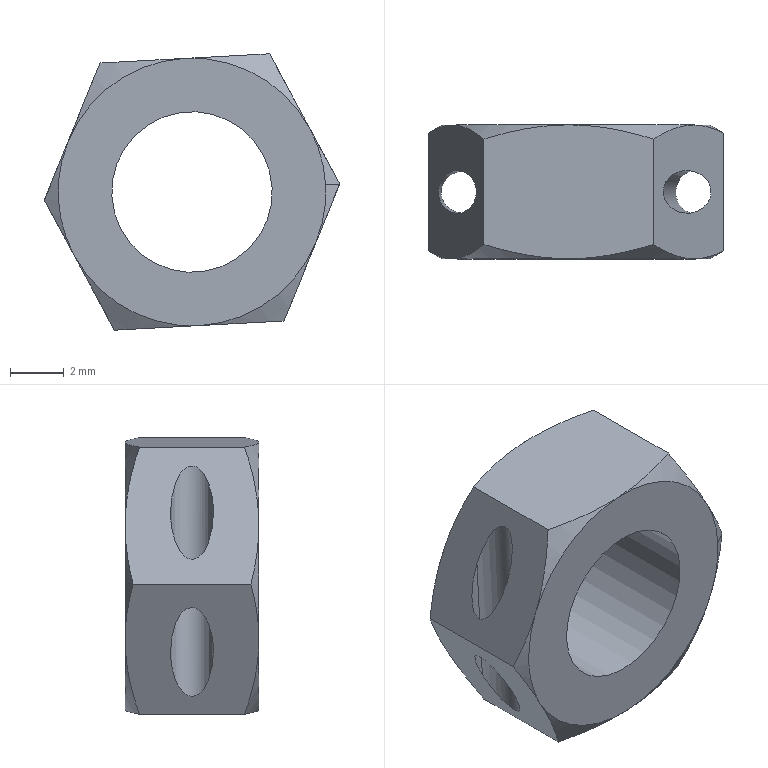Part | SolidWorks | features BaseBody 1 | 1 solid | 30 faces | box 11.034 x 5 x 10.33 mm | volume 267.643 mm3 | cone 16 | plane 8 | cylinder 6 | commonest cylinder face diameters 1.6 x4 6 x2
STEP:
#1=CARTESIAN_POINT('',(303.735,265.5,-2.369));
#2=VERTEX_POINT('',#1);
#3=CARTESIAN_POINT('',(303.735,267.1,-2.369));
#4=VERTEX_POINT('',#3);
#5=CARTESIAN_POINT('',(303.735,265.5,-2.369));
#6=CARTESIAN_POINT('',(305.148,265.5,1.117));
#7=CARTESIAN_POINT('',(305.148,267.1,1.117));
#8=CARTESIAN_POINT('',(303.735,267.1,-2.369));
#9=(BOUNDED_CURVE()B_SPLINE_CURVE(3,(#5,#6,#7,#8),.UNSPECIFIED.,.F.,.F.)B_SPLINE_CURVE_WITH_KNOTS((4,4),(4.712,7.854),.UNSPECIFIED.)CURVE()GEOMETRIC_REPRESENTATION_ITEM()RATIONAL_B_SPLINE_CURVE((1.,0.3333,0.3333,1.))REPRESENTATION_ITEM(''));
#10=EDGE_CURVE('',#2,#4,#9,.T.);
#11=ORIENTED_EDGE('',*,*,#10,.F.);
#12=CARTESIAN_POINT('',(303.452,265.5,2.835));
#13=VERTEX_POINT('',#12);
#14=CARTESIAN_POINT('',(303.865,265.5,-4.759));
#15=DIRECTION('',(-0.05426,0.,0.9985));
#16=VECTOR('',#15,1000.);
#17=LINE('',#14,#16);
#18=EDGE_CURVE('',#2,#13,#17,.T.);
#19=ORIENTED_EDGE('',*,*,#18,.T.);
#20=CARTESIAN_POINT('',(303.452,267.1,2.835));
#21=VERTEX_POINT('',#20);
#22=CARTESIAN_POINT('',(303.452,267.1,2.835));
#23=CARTESIAN_POINT('',(305.235,267.1,-0.4764));
#24=CARTESIAN_POINT('',(305.235,265.5,-0.4764));
#25=CARTESIAN_POINT('',(303.452,265.5,2.835));
#26=(BOUNDED_CURVE()B_SPLINE_CURVE(3,(#22,#23,#24,#25),.UNSPECIFIED.,.F.,.F.)B_SPLINE_CURVE_WITH_KNOTS((4,4),(1.571,4.712),.UNSPECIFIED.)CURVE()GEOMETRIC_REPRESENTATION_ITEM()RATIONAL_B_SPLINE_CURVE((1.,0.3333,0.3333,1.))REPRESENTATION_ITEM(''));
#27=EDGE_CURVE('',#21,#13,#26,.T.);
#28=ORIENTED_EDGE('',*,*,#27,.F.);
#29=CARTESIAN_POINT('',(303.865,267.1,-4.759));
#30=DIRECTION('',(-0.05426,0.,0.9985));
#31=VECTOR('',#30,1000.);
#32=LINE('',#29,#31);
#33=EDGE_CURVE('',#4,#21,#32,.T.);
#34=ORIENTED_EDGE('',*,*,#33,.F.);
#35=EDGE_LOOP('',(#11,#19,#28,#34));
#36=FACE_OUTER_BOUND('',#35,.T.);
#37=CARTESIAN_POINT('',(303.865,266.3,-4.759));
#38=DIRECTION('',(-0.05426,0.,0.9985));
#39=DIRECTION('',(0.,1.,0.));
#40=AXIS2_PLACEMENT_3D('',#37,#38,#39);
#41=CYLINDRICAL_SURFACE('',#40,0.8);
#42=ADVANCED_FACE('',(#36),#41,.F.);
#43=CARTESIAN_POINT('',(295.148,265.5,-2.835));
#44=VERTEX_POINT('',#43);
#45=CARTESIAN_POINT('',(295.148,267.1,-2.835));
#46=VERTEX_POINT('',#45);
#47=CARTESIAN_POINT('',(295.148,265.5,-2.835));
#48=CARTESIAN_POINT('',(296.93,265.5,-6.147));
#49=CARTESIAN_POINT('',(296.93,267.1,-6.147));
#50=CARTESIAN_POINT('',(295.148,267.1,-2.835));
#51=(BOUNDED_CURVE()B_SPLINE_CURVE(3,(#47,#48,#49,#50),.UNSPECIFIED.,.F.,.F.)B_SPLINE_CURVE_WITH_KNOTS((4,4),(1.571,4.712),.UNSPECIFIED.)CURVE()GEOMETRIC_REPRESENTATION_ITEM()RATIONAL_B_SPLINE_CURVE((1.,0.3333,0.3333,1.))REPRESENTATION_ITEM(''));
#52=EDGE_CURVE('',#44,#46,#51,.T.);
#53=ORIENTED_EDGE('',*,*,#52,.F.);
#54=CARTESIAN_POINT('',(294.865,265.5,2.369));
#55=VERTEX_POINT('',#54);
#56=CARTESIAN_POINT('',(295.278,265.5,-5.226));
#57=DIRECTION('',(-0.05426,0.,0.9985));
#58=VECTOR('',#57,1000.);
#59=LINE('',#56,#58);
#60=EDGE_CURVE('',#44,#55,#59,.T.);
#61=ORIENTED_EDGE('',*,*,#60,.T.);
#62=CARTESIAN_POINT('',(294.865,267.1,2.369));
#63=VERTEX_POINT('',#62);
#64=CARTESIAN_POINT('',(294.865,267.1,2.369));
#65=CARTESIAN_POINT('',(296.278,267.1,5.854));
#66=CARTESIAN_POINT('',(296.278,265.5,5.854));
#67=CARTESIAN_POINT('',(294.865,265.5,2.369));
#68=(BOUNDED_CURVE()B_SPLINE_CURVE(3,(#64,#65,#66,#67),.UNSPECIFIED.,.F.,.F.)B_SPLINE_CURVE_WITH_KNOTS((4,4),(4.712,7.854),.UNSPECIFIED.)CURVE()GEOMETRIC_REPRESENTATION_ITEM()RATIONAL_B_SPLINE_CURVE((1.,0.3333,0.3333,1.))REPRESENTATION_ITEM(''));
#69=EDGE_CURVE('',#63,#55,#68,.T.);
#70=ORIENTED_EDGE('',*,*,#69,.F.);
#71=CARTESIAN_POINT('',(295.278,267.1,-5.226));
#72=DIRECTION('',(-0.05426,0.,0.9985));
#73=VECTOR('',#72,1000.);
#74=LINE('',#71,#73);
#75=EDGE_CURVE('',#46,#63,#74,.T.);
#76=ORIENTED_EDGE('',*,*,#75,.F.);
#77=EDGE_LOOP('',(#53,#61,#70,#76));
#78=FACE_OUTER_BOUND('',#77,.T.);
#79=CARTESIAN_POINT('',(295.278,266.3,-5.226));
#80=DIRECTION('',(-0.05426,0.,0.9985));
#81=DIRECTION('',(0.,1.,0.));
#82=AXIS2_PLACEMENT_3D('',#79,#80,#81);
#83=CYLINDRICAL_SURFACE('',#82,0.8);
#84=ADVANCED_FACE('',(#78),#83,.F.);
#85=CARTESIAN_POINT('',(302.296,268.3,0.1628));
#86=VERTEX_POINT('',#85);
#87=CARTESIAN_POINT('',(296.304,268.3,-0.1628));
#88=VERTEX_POINT('',#87);
#89=CARTESIAN_POINT('',(299.3,268.3,0.));
#90=DIRECTION('',(0.,1.,0.));
#91=DIRECTION('',(0.9985,0.,0.05426));
#92=AXIS2_PLACEMENT_3D('',#89,#90,#91);
#93=CIRCLE('',#92,3.);
#94=EDGE_CURVE('',#86,#88,#93,.T.);
#95=ORIENTED_EDGE('',*,*,#94,.F.);
#96=CARTESIAN_POINT('',(302.795,268.8,0.1899));
#97=VERTEX_POINT('',#96);
#98=CARTESIAN_POINT('',(302.296,268.3,0.1628));
#99=DIRECTION('',(0.7061,0.7071,0.03836));
#100=VECTOR('',#99,1000.);
#101=LINE('',#98,#100);
#102=EDGE_CURVE('',#86,#97,#101,.T.);
#103=ORIENTED_EDGE('',*,*,#102,.T.);
#104=CARTESIAN_POINT('',(295.805,268.8,-0.1899));
#105=VERTEX_POINT('',#104);
#106=CARTESIAN_POINT('',(299.3,268.8,0.));
#107=DIRECTION('',(0.,-1.,0.));
#108=DIRECTION('',(0.9985,0.,0.05426));
#109=AXIS2_PLACEMENT_3D('',#106,#107,#108);
#110=CIRCLE('',#109,3.5);
#111=EDGE_CURVE('',#105,#97,#110,.T.);
#112=ORIENTED_EDGE('',*,*,#111,.F.);
#113=CARTESIAN_POINT('',(296.304,268.3,-0.1628));
#114=DIRECTION('',(-0.7061,0.7071,-0.03836));
#115=VECTOR('',#114,1000.);
#116=LINE('',#113,#115);
#117=EDGE_CURVE('',#88,#105,#116,.T.);
#118=ORIENTED_EDGE('',*,*,#117,.F.);
#119=EDGE_LOOP('',(#95,#103,#112,#118));
#120=FACE_OUTER_BOUND('',#119,.T.);
#121=CARTESIAN_POINT('',(299.3,268.3,0.));
#122=DIRECTION('',(0.,1.,0.));
#123=DIRECTION('',(-0.9985,0.,-0.05426));
#124=AXIS2_PLACEMENT_3D('',#121,#122,#123);
#125=CONICAL_SURFACE('',#124,3.,0.7854);
#126=ADVANCED_FACE('',(#120),#125,.F.);
#127=CARTESIAN_POINT('',(296.304,263.8,-0.1628));
#128=VERTEX_POINT('',#127);
#129=CARTESIAN_POINT('',(302.296,263.8,0.1628));
#130=VERTEX_POINT('',#129);
#131=CARTESIAN_POINT('',(299.3,263.8,0.));
#132=DIRECTION('',(0.,-1.,0.));
#133=DIRECTION('',(0.9985,0.,0.05426));
#134=AXIS2_PLACEMENT_3D('',#131,#132,#133);
#135=CIRCLE('',#134,3.);
#136=EDGE_CURVE('',#128,#130,#135,.T.);
#137=ORIENTED_EDGE('',*,*,#136,.T.);
#138=CARTESIAN_POINT('',(302.296,258.8,0.1628));
#139=DIRECTION('',(0.,1.,0.));
#140=VECTOR('',#139,1000.);
#141=LINE('',#138,#140);
#142=EDGE_CURVE('',#130,#86,#141,.T.);
#143=ORIENTED_EDGE('',*,*,#142,.T.);
#144=ORIENTED_EDGE('',*,*,#94,.T.);
#145=CARTESIAN_POINT('',(296.304,258.8,-0.1628));
#146=DIRECTION('',(0.,1.,0.));
#147=VECTOR('',#146,1000.);
#148=LINE('',#145,#147);
#149=EDGE_CURVE('',#128,#88,#148,.T.);
#150=ORIENTED_EDGE('',*,*,#149,.F.);
#151=EDGE_LOOP('',(#137,#143,#144,#150));
#152=FACE_OUTER_BOUND('',#151,.T.);
#153=CARTESIAN_POINT('',(299.3,258.8,0.));
#154=DIRECTION('',(0.,1.,0.));
#155=DIRECTION('',(-0.9985,0.,-0.05426));
#156=AXIS2_PLACEMENT_3D('',#153,#154,#155);
#157=CYLINDRICAL_SURFACE('',#156,3.);
#158=ADVANCED_FACE('',(#152),#157,.F.);
#159=CARTESIAN_POINT('',(303.703,263.8,2.37));
#160=VERTEX_POINT('',#159);
#161=CARTESIAN_POINT('',(304.293,263.8,0.2713));
#162=VERTEX_POINT('',#161);
#163=CARTESIAN_POINT('',(299.3,263.8,0.));
#164=DIRECTION('',(0.,1.,0.));
#165=DIRECTION('',(0.9985,0.,0.05426));
#166=AXIS2_PLACEMENT_3D('',#163,#164,#165);
#167=CIRCLE('',#166,5.);
#168=EDGE_CURVE('',#160,#162,#167,.T.);
#169=ORIENTED_EDGE('',*,*,#168,.T.);
#170=CARTESIAN_POINT('',(304.817,264.103,0.2998));
#171=VERTEX_POINT('',#170);
#172=CARTESIAN_POINT('',(304.293,263.8,0.2713));
#173=DIRECTION('',(0.8647,0.5,0.04699));
#174=VECTOR('',#173,1000.);
#175=LINE('',#172,#174);
#176=EDGE_CURVE('',#162,#171,#175,.T.);
#177=ORIENTED_EDGE('',*,*,#176,.T.);
#178=CARTESIAN_POINT('',(304.817,264.103,0.2998));
#179=CARTESIAN_POINT('',(304.449,263.913,0.9823));
#180=CARTESIAN_POINT('',(304.079,263.8,1.671));
#181=CARTESIAN_POINT('',(303.703,263.8,2.37));
#182=B_SPLINE_CURVE_WITH_KNOTS('',3,(#178,#179,#180,#181),.UNSPECIFIED.,.F.,.F.,(4,4),(0.000000225,0.002369),.UNSPECIFIED.);
#183=EDGE_CURVE('',#171,#160,#182,.T.);
#184=ORIENTED_EDGE('',*,*,#183,.T.);
#185=EDGE_LOOP('',(#169,#177,#184));
#186=FACE_OUTER_BOUND('',#185,.T.);
#187=CARTESIAN_POINT('',(299.3,263.8,0.));
#188=DIRECTION('',(0.,1.,0.));
#189=DIRECTION('',(0.9985,0.,0.05426));
#190=AXIS2_PLACEMENT_3D('',#187,#188,#189);
#191=CONICAL_SURFACE('',#190,5.,1.047);
#192=ADVANCED_FACE('',(#186),#191,.T.);
#193=CARTESIAN_POINT('',(294.307,268.8,-0.2713));
#194=VERTEX_POINT('',#193);
#195=CARTESIAN_POINT('',(294.666,268.8,1.879));
#196=VERTEX_POINT('',#195);
#197=CARTESIAN_POINT('',(299.3,268.8,0.));
#198=DIRECTION('',(0.,1.,0.));
#199=DIRECTION('',(0.9985,0.,0.05426));
#200=AXIS2_PLACEMENT_3D('',#197,#198,#199);
#201=CIRCLE('',#200,5.);
#202=EDGE_CURVE('',#194,#196,#201,.T.);
#203=ORIENTED_EDGE('',*,*,#202,.F.);
#204=CARTESIAN_POINT('',(293.783,268.497,-0.2998));
#205=VERTEX_POINT('',#204);
#206=CARTESIAN_POINT('',(294.307,268.8,-0.2713));
#207=DIRECTION('',(-0.8647,-0.5,-0.04699));
#208=VECTOR('',#207,1000.);
#209=LINE('',#206,#208);
#210=EDGE_CURVE('',#194,#205,#209,.T.);
#211=ORIENTED_EDGE('',*,*,#210,.T.);
#212=CARTESIAN_POINT('',(293.783,268.497,-0.2998));
#213=CARTESIAN_POINT('',(294.074,268.687,0.4186));
#214=CARTESIAN_POINT('',(294.368,268.8,1.144));
#215=CARTESIAN_POINT('',(294.666,268.8,1.879));
#216=B_SPLINE_CURVE_WITH_KNOTS('',3,(#212,#213,#214,#215),.UNSPECIFIED.,.F.,.F.,(4,4),(0.000000225,0.002369),.UNSPECIFIED.);
#217=EDGE_CURVE('',#205,#196,#216,.T.);
#218=ORIENTED_EDGE('',*,*,#217,.T.);
#219=EDGE_LOOP('',(#203,#211,#218));
#220=FACE_OUTER_BOUND('',#219,.T.);
#221=CARTESIAN_POINT('',(299.3,268.8,0.));
#222=DIRECTION('',(0.,-1.,0.));
#223=DIRECTION('',(-0.9985,0.,-0.05426));
#224=AXIS2_PLACEMENT_3D('',#221,#222,#223);
#225=CONICAL_SURFACE('',#224,5.,1.047);
#226=ADVANCED_FACE('',(#220),#225,.T.);
#227=CARTESIAN_POINT('',(295.148,267.1,-2.835));
#228=CARTESIAN_POINT('',(293.365,267.1,0.4764));
#229=CARTESIAN_POINT('',(293.365,265.5,0.4764));
#230=CARTESIAN_POINT('',(295.148,265.5,-2.835));
#231=(BOUNDED_CURVE()B_SPLINE_CURVE(3,(#227,#228,#229,#230),.UNSPECIFIED.,.F.,.F.)B_SPLINE_CURVE_WITH_KNOTS((4,4),(4.712,7.854),.UNSPECIFIED.)CURVE()GEOMETRIC_REPRESENTATION_ITEM()RATIONAL_B_SPLINE_CURVE((1.,0.3333,0.3333,1.))REPRESENTATION_ITEM(''));
#232=EDGE_CURVE('',#46,#44,#231,.T.);
#233=ORIENTED_EDGE('',*,*,#232,.T.);
#234=ORIENTED_EDGE('',*,*,#52,.T.);
#235=EDGE_LOOP('',(#233,#234));
#236=FACE_BOUND('',#235,.T.);
#237=CARTESIAN_POINT('',(293.783,264.103,-0.2998));
#238=VERTEX_POINT('',#237);
#239=CARTESIAN_POINT('',(294.897,263.8,-2.37));
#240=VERTEX_POINT('',#239);
#241=CARTESIAN_POINT('',(293.783,264.103,-0.2998));
#242=CARTESIAN_POINT('',(294.151,263.913,-0.9823));
#243=CARTESIAN_POINT('',(294.521,263.8,-1.671));
#244=CARTESIAN_POINT('',(294.897,263.8,-2.37));
#245=B_SPLINE_CURVE_WITH_KNOTS('',3,(#241,#242,#243,#244),.UNSPECIFIED.,.F.,.F.,(4,4),(0.000000225,0.002369),.UNSPECIFIED.);
#246=EDGE_CURVE('',#238,#240,#245,.T.);
#247=ORIENTED_EDGE('',*,*,#246,.F.);
#248=CARTESIAN_POINT('',(293.783,268.8,-0.2998));
#249=DIRECTION('',(0.,-1.,0.));
#250=VECTOR('',#249,1000.);
#251=LINE('',#248,#250);
#252=EDGE_CURVE('',#205,#238,#251,.T.);
#253=ORIENTED_EDGE('',*,*,#252,.F.);
#254=CARTESIAN_POINT('',(294.897,268.8,-2.37));
#255=VERTEX_POINT('',#254);
#256=CARTESIAN_POINT('',(294.897,268.8,-2.37));
#257=CARTESIAN_POINT('',(294.52,268.8,-1.668));
#258=CARTESIAN_POINT('',(294.149,268.687,-0.9797));
#259=CARTESIAN_POINT('',(293.783,268.497,-0.2998));
#260=B_SPLINE_CURVE_WITH_KNOTS('',3,(#256,#257,#258,#259),.UNSPECIFIED.,.F.,.F.,(4,4),(0.003219,0.005576),.UNSPECIFIED.);
#261=EDGE_CURVE('',#255,#205,#260,.T.);
#262=ORIENTED_EDGE('',*,*,#261,.F.);
#263=CARTESIAN_POINT('',(296.402,268.267,-5.165));
#264=VERTEX_POINT('',#263);
#265=CARTESIAN_POINT('',(296.402,268.267,-5.165));
#266=CARTESIAN_POINT('',(295.912,268.587,-4.254));
#267=CARTESIAN_POINT('',(295.413,268.8,-3.327));
#268=CARTESIAN_POINT('',(294.897,268.8,-2.37));
#269=B_SPLINE_CURVE_WITH_KNOTS('',3,(#265,#266,#267,#268),.UNSPECIFIED.,.F.,.F.,(4,4),(0.000000229,0.003219),.UNSPECIFIED.);
#270=EDGE_CURVE('',#264,#255,#269,.T.);
#271=ORIENTED_EDGE('',*,*,#270,.F.);
#272=CARTESIAN_POINT('',(296.402,264.333,-5.165));
#273=VERTEX_POINT('',#272);
#274=CARTESIAN_POINT('',(296.402,268.8,-5.165));
#275=DIRECTION('',(0.,-1.,0.));
#276=VECTOR('',#275,1000.);
#277=LINE('',#274,#276);
#278=EDGE_CURVE('',#264,#273,#277,.T.);
#279=ORIENTED_EDGE('',*,*,#278,.T.);
#280=CARTESIAN_POINT('',(294.897,263.8,-2.37));
#281=CARTESIAN_POINT('',(295.024,263.8,-2.606));
#282=CARTESIAN_POINT('',(295.153,263.813,-2.844));
#283=CARTESIAN_POINT('',(295.408,263.862,-3.318));
#284=CARTESIAN_POINT('',(295.534,263.899,-3.553));
#285=CARTESIAN_POINT('',(295.91,264.039,-4.252));
#286=CARTESIAN_POINT('',(296.157,264.173,-4.711));
#287=CARTESIAN_POINT('',(296.402,264.333,-5.165));
#288=B_SPLINE_CURVE_WITH_KNOTS('',3,(#280,#281,#282,#283,#284,#285,#286,#287),.UNSPECIFIED.,.F.,.F.,(4,2,2,4),(0.002369,0.00317,0.003971,0.005574),.UNSPECIFIED.);
#289=EDGE_CURVE('',#240,#273,#288,.T.);
#290=ORIENTED_EDGE('',*,*,#289,.F.);
#291=EDGE_LOOP('',(#247,#253,#262,#271,#279,#290));
#292=FACE_OUTER_BOUND('',#291,.T.);
#293=CARTESIAN_POINT('',(296.402,268.8,-5.165));
#294=DIRECTION('',(0.8806,0.,0.4739));
#295=DIRECTION('',(0.4739,0.,-0.8806));
#296=AXIS2_PLACEMENT_3D('',#293,#294,#295);
#297=PLANE('',#296);
#298=ADVANCED_FACE('',(#236,#292),#297,.F.);
#299=ORIENTED_EDGE('',*,*,#69,.T.);
#300=CARTESIAN_POINT('',(294.865,265.5,2.369));
#301=CARTESIAN_POINT('',(293.452,265.5,-1.117));
#302=CARTESIAN_POINT('',(293.452,267.1,-1.117));
#303=CARTESIAN_POINT('',(294.865,267.1,2.369));
#304=(BOUNDED_CURVE()B_SPLINE_CURVE(3,(#300,#301,#302,#303),.UNSPECIFIED.,.F.,.F.)B_SPLINE_CURVE_WITH_KNOTS((4,4),(1.571,4.712),.UNSPECIFIED.)CURVE()GEOMETRIC_REPRESENTATION_ITEM()RATIONAL_B_SPLINE_CURVE((1.,0.3333,0.3333,1.))REPRESENTATION_ITEM(''));
#305=EDGE_CURVE('',#55,#63,#304,.T.);
#306=ORIENTED_EDGE('',*,*,#305,.T.);
#307=EDGE_LOOP('',(#299,#306));
#308=FACE_BOUND('',#307,.T.);
#309=CARTESIAN_POINT('',(295.859,264.333,4.82));
#310=VERTEX_POINT('',#309);
#311=CARTESIAN_POINT('',(294.666,263.8,1.879));
#312=VERTEX_POINT('',#311);
#313=CARTESIAN_POINT('',(295.859,264.333,4.82));
#314=CARTESIAN_POINT('',(295.471,264.013,3.862));
#315=CARTESIAN_POINT('',(295.075,263.8,2.886));
#316=CARTESIAN_POINT('',(294.666,263.8,1.879));
#317=B_SPLINE_CURVE_WITH_KNOTS('',3,(#313,#314,#315,#316),.UNSPECIFIED.,.F.,.F.,(4,4),(0.000000229,0.003219),.UNSPECIFIED.);
#318=EDGE_CURVE('',#310,#312,#317,.T.);
#319=ORIENTED_EDGE('',*,*,#318,.F.);
#320=CARTESIAN_POINT('',(295.859,268.267,4.82));
#321=VERTEX_POINT('',#320);
#322=CARTESIAN_POINT('',(295.859,268.8,4.82));
#323=DIRECTION('',(0.,-1.,0.));
#324=VECTOR('',#323,1000.);
#325=LINE('',#322,#324);
#326=EDGE_CURVE('',#321,#310,#325,.T.);
#327=ORIENTED_EDGE('',*,*,#326,.F.);
#328=CARTESIAN_POINT('',(294.666,268.8,1.879));
#329=CARTESIAN_POINT('',(294.767,268.8,2.127));
#330=CARTESIAN_POINT('',(294.869,268.787,2.378));
#331=CARTESIAN_POINT('',(295.071,268.738,2.877));
#332=CARTESIAN_POINT('',(295.171,268.701,3.124));
#333=CARTESIAN_POINT('',(295.469,268.561,3.859));
#334=CARTESIAN_POINT('',(295.665,268.427,4.342));
#335=CARTESIAN_POINT('',(295.859,268.267,4.82));
#336=B_SPLINE_CURVE_WITH_KNOTS('',3,(#328,#329,#330,#331,#332,#333,#334,#335),.UNSPECIFIED.,.F.,.F.,(4,2,2,4),(0.002369,0.00317,0.003971,0.005574),.UNSPECIFIED.);
#337=EDGE_CURVE('',#196,#321,#336,.T.);
#338=ORIENTED_EDGE('',*,*,#337,.F.);
#339=ORIENTED_EDGE('',*,*,#217,.F.);
#340=ORIENTED_EDGE('',*,*,#252,.T.);
#341=CARTESIAN_POINT('',(294.666,263.8,1.879));
#342=CARTESIAN_POINT('',(294.367,263.8,1.141));
#343=CARTESIAN_POINT('',(294.073,263.913,0.4159));
#344=CARTESIAN_POINT('',(293.783,264.103,-0.2998));
#345=B_SPLINE_CURVE_WITH_KNOTS('',3,(#341,#342,#343,#344),.UNSPECIFIED.,.F.,.F.,(4,4),(0.003219,0.005576),.UNSPECIFIED.);
#346=EDGE_CURVE('',#312,#238,#345,.T.);
#347=ORIENTED_EDGE('',*,*,#346,.F.);
#348=EDGE_LOOP('',(#319,#327,#338,#339,#340,#347));
#349=FACE_OUTER_BOUND('',#348,.T.);
#350=CARTESIAN_POINT('',(295.859,268.8,4.82));
#351=DIRECTION('',(0.9267,0.,-0.3757));
#352=DIRECTION('',(-0.3757,0.,-0.9267));
#353=AXIS2_PLACEMENT_3D('',#350,#351,#352);
#354=PLANE('',#353);
#355=ADVANCED_FACE('',(#308,#349),#354,.F.);
#356=CARTESIAN_POINT('',(302.198,264.333,5.165));
#357=VERTEX_POINT('',#356);
#358=CARTESIAN_POINT('',(299.029,263.8,4.993));
#359=VERTEX_POINT('',#358);
#360=CARTESIAN_POINT('',(302.198,264.333,5.165));
#361=CARTESIAN_POINT('',(301.684,264.173,5.137));
#362=CARTESIAN_POINT('',(301.158,264.038,5.108));
#363=CARTESIAN_POINT('',(300.101,263.851,5.051));
#364=CARTESIAN_POINT('',(299.568,263.8,5.022));
#365=CARTESIAN_POINT('',(299.029,263.8,4.993));
#366=B_SPLINE_CURVE_WITH_KNOTS('',3,(#360,#361,#362,#363,#364,#365),.UNSPECIFIED.,.F.,.F.,(4,2,4),(0.005496,0.007108,0.008721),.UNSPECIFIED.);
#367=EDGE_CURVE('',#357,#359,#366,.T.);
#368=ORIENTED_EDGE('',*,*,#367,.F.);
#369=CARTESIAN_POINT('',(302.198,268.267,5.165));
#370=VERTEX_POINT('',#369);
#371=CARTESIAN_POINT('',(302.198,268.8,5.165));
#372=DIRECTION('',(0.,-1.,0.));
#373=VECTOR('',#372,1000.);
#374=LINE('',#371,#373);
#375=EDGE_CURVE('',#370,#357,#374,.T.);
#376=ORIENTED_EDGE('',*,*,#375,.F.);
#377=CARTESIAN_POINT('',(299.029,268.8,4.993));
#378=VERTEX_POINT('',#377);
#379=CARTESIAN_POINT('',(299.029,268.8,4.993));
#380=CARTESIAN_POINT('',(299.568,268.8,5.022));
#381=CARTESIAN_POINT('',(300.101,268.749,5.051));
#382=CARTESIAN_POINT('',(301.158,268.562,5.108));
#383=CARTESIAN_POINT('',(301.684,268.427,5.137));
#384=CARTESIAN_POINT('',(302.198,268.267,5.165));
#385=B_SPLINE_CURVE_WITH_KNOTS('',3,(#379,#380,#381,#382,#383,#384),.UNSPECIFIED.,.F.,.F.,(4,2,4),(0.01912,0.02073,0.02233),.UNSPECIFIED.);
#386=EDGE_CURVE('',#378,#370,#385,.T.);
#387=ORIENTED_EDGE('',*,*,#386,.F.);
#388=CARTESIAN_POINT('',(295.859,268.267,4.82));
#389=CARTESIAN_POINT('',(296.373,268.427,4.848));
#390=CARTESIAN_POINT('',(296.892,268.56,4.877));
#391=CARTESIAN_POINT('',(297.684,268.701,4.92));
#392=CARTESIAN_POINT('',(297.95,268.737,4.934));
#393=CARTESIAN_POINT('',(298.487,268.787,4.963));
#394=CARTESIAN_POINT('',(298.759,268.8,4.978));
#395=CARTESIAN_POINT('',(299.029,268.8,4.993));
#396=B_SPLINE_CURVE_WITH_KNOTS('',3,(#388,#389,#390,#391,#392,#393,#394,#395),.UNSPECIFIED.,.F.,.F.,(4,2,2,4),(0.0159,0.01751,0.01831,0.01912),.UNSPECIFIED.);
#397=EDGE_CURVE('',#321,#378,#396,.T.);
#398=ORIENTED_EDGE('',*,*,#397,.F.);
#399=ORIENTED_EDGE('',*,*,#326,.T.);
#400=CARTESIAN_POINT('',(299.029,263.8,4.993));
#401=CARTESIAN_POINT('',(298.759,263.8,4.978));
#402=CARTESIAN_POINT('',(298.487,263.813,4.963));
#403=CARTESIAN_POINT('',(297.95,263.863,4.934));
#404=CARTESIAN_POINT('',(297.684,263.899,4.92));
#405=CARTESIAN_POINT('',(296.892,264.04,4.877));
#406=CARTESIAN_POINT('',(296.373,264.173,4.848));
#407=CARTESIAN_POINT('',(295.859,264.333,4.82));
#408=B_SPLINE_CURVE_WITH_KNOTS('',3,(#400,#401,#402,#403,#404,#405,#406,#407),.UNSPECIFIED.,.F.,.F.,(4,2,2,4),(0.008721,0.009526,0.01033,0.01194),.UNSPECIFIED.);
#409=EDGE_CURVE('',#359,#310,#408,.T.);
#410=ORIENTED_EDGE('',*,*,#409,.F.);
#411=EDGE_LOOP('',(#368,#376,#387,#398,#399,#410));
#412=FACE_OUTER_BOUND('',#411,.T.);
#413=CARTESIAN_POINT('',(302.198,268.8,5.165));
#414=DIRECTION('',(0.05426,0.,-0.9985));
#415=DIRECTION('',(0.,-1.,0.));
#416=AXIS2_PLACEMENT_3D('',#413,#414,#415);
#417=PLANE('',#416);
#418=ADVANCED_FACE('',(#412),#417,.F.);
#419=ORIENTED_EDGE('',*,*,#27,.T.);
#420=CARTESIAN_POINT('',(303.452,265.5,2.835));
#421=CARTESIAN_POINT('',(301.67,265.5,6.147));
#422=CARTESIAN_POINT('',(301.67,267.1,6.147));
#423=CARTESIAN_POINT('',(303.452,267.1,2.835));
#424=(BOUNDED_CURVE()B_SPLINE_CURVE(3,(#420,#421,#422,#423),.UNSPECIFIED.,.F.,.F.)B_SPLINE_CURVE_WITH_KNOTS((4,4),(4.712,7.854),.UNSPECIFIED.)CURVE()GEOMETRIC_REPRESENTATION_ITEM()RATIONAL_B_SPLINE_CURVE((1.,0.3333,0.3333,1.))REPRESENTATION_ITEM(''));
#425=EDGE_CURVE('',#13,#21,#424,.T.);
#426=ORIENTED_EDGE('',*,*,#425,.T.);
#427=EDGE_LOOP('',(#419,#426));
#428=FACE_BOUND('',#427,.T.);
#429=ORIENTED_EDGE('',*,*,#183,.F.);
#430=CARTESIAN_POINT('',(304.817,268.497,0.2998));
#431=VERTEX_POINT('',#430);
#432=CARTESIAN_POINT('',(304.817,268.8,0.2998));
#433=DIRECTION('',(0.,-1.,0.));
#434=VECTOR('',#433,1000.);
#435=LINE('',#432,#434);
#436=EDGE_CURVE('',#431,#171,#435,.T.);
#437=ORIENTED_EDGE('',*,*,#436,.F.);
#438=CARTESIAN_POINT('',(303.703,268.8,2.37));
#439=VERTEX_POINT('',#438);
#440=CARTESIAN_POINT('',(303.703,268.8,2.37));
#441=CARTESIAN_POINT('',(304.08,268.8,1.668));
#442=CARTESIAN_POINT('',(304.451,268.687,0.9797));
#443=CARTESIAN_POINT('',(304.817,268.497,0.2998));
#444=B_SPLINE_CURVE_WITH_KNOTS('',3,(#440,#441,#442,#443),.UNSPECIFIED.,.F.,.F.,(4,4),(0.003219,0.005576),.UNSPECIFIED.);
#445=EDGE_CURVE('',#439,#431,#444,.T.);
#446=ORIENTED_EDGE('',*,*,#445,.F.);
#447=CARTESIAN_POINT('',(302.198,268.267,5.165));
#448=CARTESIAN_POINT('',(302.688,268.587,4.254));
#449=CARTESIAN_POINT('',(303.187,268.8,3.327));
#450=CARTESIAN_POINT('',(303.703,268.8,2.37));
#451=B_SPLINE_CURVE_WITH_KNOTS('',3,(#447,#448,#449,#450),.UNSPECIFIED.,.F.,.F.,(4,4),(0.000000229,0.003219),.UNSPECIFIED.);
#452=EDGE_CURVE('',#370,#439,#451,.T.);
#453=ORIENTED_EDGE('',*,*,#452,.F.);
#454=ORIENTED_EDGE('',*,*,#375,.T.);
#455=CARTESIAN_POINT('',(303.703,263.8,2.37));
#456=CARTESIAN_POINT('',(303.576,263.8,2.606));
#457=CARTESIAN_POINT('',(303.447,263.813,2.844));
#458=CARTESIAN_POINT('',(303.192,263.862,3.318));
#459=CARTESIAN_POINT('',(303.066,263.899,3.553));
#460=CARTESIAN_POINT('',(302.69,264.039,4.252));
#461=CARTESIAN_POINT('',(302.443,264.173,4.711));
#462=CARTESIAN_POINT('',(302.198,264.333,5.165));
#463=B_SPLINE_CURVE_WITH_KNOTS('',3,(#455,#456,#457,#458,#459,#460,#461,#462),.UNSPECIFIED.,.F.,.F.,(4,2,2,4),(0.002369,0.00317,0.003971,0.005574),.UNSPECIFIED.);
#464=EDGE_CURVE('',#160,#357,#463,.T.);
#465=ORIENTED_EDGE('',*,*,#464,.F.);
#466=EDGE_LOOP('',(#429,#437,#446,#453,#454,#465));
#467=FACE_OUTER_BOUND('',#466,.T.);
#468=CARTESIAN_POINT('',(302.198,268.8,5.165));
#469=DIRECTION('',(-0.8806,0.,-0.4739));
#470=DIRECTION('',(-0.4739,0.,0.8806));
#471=AXIS2_PLACEMENT_3D('',#468,#469,#470);
#472=PLANE('',#471);
#473=ADVANCED_FACE('',(#428,#467),#472,.F.);
#474=CARTESIAN_POINT('',(303.735,267.1,-2.369));
#475=CARTESIAN_POINT('',(302.322,267.1,-5.854));
#476=CARTESIAN_POINT('',(302.322,265.5,-5.854));
#477=CARTESIAN_POINT('',(303.735,265.5,-2.369));
#478=(BOUNDED_CURVE()B_SPLINE_CURVE(3,(#474,#475,#476,#477),.UNSPECIFIED.,.F.,.T.)B_SPLINE_CURVE_WITH_KNOTS((4,4),(1.571,4.712),.UNSPECIFIED.)CURVE()GEOMETRIC_REPRESENTATION_ITEM()RATIONAL_B_SPLINE_CURVE((1.,0.3333,0.3333,1.))REPRESENTATION_ITEM(''));
#479=EDGE_CURVE('',#4,#2,#478,.T.);
#480=ORIENTED_EDGE('',*,*,#479,.T.);
#481=ORIENTED_EDGE('',*,*,#10,.T.);
#482=EDGE_LOOP('',(#480,#481));
#483=FACE_BOUND('',#482,.T.);
#484=CARTESIAN_POINT('',(302.741,264.333,-4.82));
#485=VERTEX_POINT('',#484);
#486=CARTESIAN_POINT('',(303.934,263.8,-1.879));
#487=VERTEX_POINT('',#486);
#488=CARTESIAN_POINT('',(302.741,264.333,-4.82));
#489=CARTESIAN_POINT('',(303.129,264.013,-3.862));
#490=CARTESIAN_POINT('',(303.525,263.8,-2.886));
#491=CARTESIAN_POINT('',(303.934,263.8,-1.879));
#492=B_SPLINE_CURVE_WITH_KNOTS('',3,(#488,#489,#490,#491),.UNSPECIFIED.,.F.,.F.,(4,4),(0.000000229,0.003219),.UNSPECIFIED.);
#493=EDGE_CURVE('',#485,#487,#492,.T.);
#494=ORIENTED_EDGE('',*,*,#493,.F.);
#495=CARTESIAN_POINT('',(302.741,268.267,-4.82));
#496=VERTEX_POINT('',#495);
#497=CARTESIAN_POINT('',(302.741,268.8,-4.82));
#498=DIRECTION('',(0.,-1.,0.));
#499=VECTOR('',#498,1000.);
#500=LINE('',#497,#499);
#501=EDGE_CURVE('',#496,#485,#500,.T.);
#502=ORIENTED_EDGE('',*,*,#501,.F.);
#503=CARTESIAN_POINT('',(303.934,268.8,-1.879));
#504=VERTEX_POINT('',#503);
#505=CARTESIAN_POINT('',(303.934,268.8,-1.879));
#506=CARTESIAN_POINT('',(303.833,268.8,-2.127));
#507=CARTESIAN_POINT('',(303.731,268.787,-2.378));
#508=CARTESIAN_POINT('',(303.529,268.738,-2.877));
#509=CARTESIAN_POINT('',(303.429,268.701,-3.124));
#510=CARTESIAN_POINT('',(303.131,268.561,-3.859));
#511=CARTESIAN_POINT('',(302.935,268.427,-4.342));
#512=CARTESIAN_POINT('',(302.741,268.267,-4.82));
#513=B_SPLINE_CURVE_WITH_KNOTS('',3,(#505,#506,#507,#508,#509,#510,#511,#512),.UNSPECIFIED.,.F.,.F.,(4,2,2,4),(0.002369,0.00317,0.003971,0.005574),.UNSPECIFIED.);
#514=EDGE_CURVE('',#504,#496,#513,.T.);
#515=ORIENTED_EDGE('',*,*,#514,.F.);
#516=CARTESIAN_POINT('',(304.817,268.497,0.2998));
#517=CARTESIAN_POINT('',(304.526,268.687,-0.4186));
#518=CARTESIAN_POINT('',(304.232,268.8,-1.144));
#519=CARTESIAN_POINT('',(303.934,268.8,-1.879));
#520=B_SPLINE_CURVE_WITH_KNOTS('',3,(#516,#517,#518,#519),.UNSPECIFIED.,.F.,.F.,(4,4),(0.000000225,0.002369),.UNSPECIFIED.);
#521=EDGE_CURVE('',#431,#504,#520,.T.);
#522=ORIENTED_EDGE('',*,*,#521,.F.);
#523=ORIENTED_EDGE('',*,*,#436,.T.);
#524=CARTESIAN_POINT('',(303.934,263.8,-1.879));
#525=CARTESIAN_POINT('',(304.233,263.8,-1.141));
#526=CARTESIAN_POINT('',(304.527,263.913,-0.4159));
#527=CARTESIAN_POINT('',(304.817,264.103,0.2998));
#528=B_SPLINE_CURVE_WITH_KNOTS('',3,(#524,#525,#526,#527),.UNSPECIFIED.,.F.,.F.,(4,4),(0.003219,0.005576),.UNSPECIFIED.);
#529=EDGE_CURVE('',#487,#171,#528,.T.);
#530=ORIENTED_EDGE('',*,*,#529,.F.);
#531=EDGE_LOOP('',(#494,#502,#515,#522,#523,#530));
#532=FACE_OUTER_BOUND('',#531,.T.);
#533=CARTESIAN_POINT('',(302.741,268.8,-4.82));
#534=DIRECTION('',(-0.9267,0.,0.3757));
#535=DIRECTION('',(0.3757,0.,0.9267));
#536=AXIS2_PLACEMENT_3D('',#533,#534,#535);
#537=PLANE('',#536);
#538=ADVANCED_FACE('',(#483,#532),#537,.F.);
#539=CARTESIAN_POINT('',(299.571,263.8,-4.993));
#540=VERTEX_POINT('',#539);
#541=CARTESIAN_POINT('',(296.402,264.333,-5.165));
#542=CARTESIAN_POINT('',(296.916,264.173,-5.137));
#543=CARTESIAN_POINT('',(297.435,264.04,-5.109));
#544=CARTESIAN_POINT('',(298.227,263.899,-5.066));
#545=CARTESIAN_POINT('',(298.493,263.863,-5.051));
#546=CARTESIAN_POINT('',(299.03,263.813,-5.022));
#547=CARTESIAN_POINT('',(299.302,263.8,-5.007));
#548=CARTESIAN_POINT('',(299.571,263.8,-4.993));
#549=B_SPLINE_CURVE_WITH_KNOTS('',3,(#541,#542,#543,#544,#545,#546,#547,#548),.UNSPECIFIED.,.F.,.F.,(4,2,2,4),(0.0159,0.01751,0.01831,0.01912),.UNSPECIFIED.);
#550=EDGE_CURVE('',#273,#540,#549,.T.);
#551=ORIENTED_EDGE('',*,*,#550,.F.);
#552=ORIENTED_EDGE('',*,*,#278,.F.);
#553=CARTESIAN_POINT('',(299.571,268.8,-4.993));
#554=VERTEX_POINT('',#553);
#555=CARTESIAN_POINT('',(299.571,268.8,-4.993));
#556=CARTESIAN_POINT('',(299.302,268.8,-5.007));
#557=CARTESIAN_POINT('',(299.03,268.787,-5.022));
#558=CARTESIAN_POINT('',(298.493,268.737,-5.051));
#559=CARTESIAN_POINT('',(298.227,268.701,-5.066));
#560=CARTESIAN_POINT('',(297.435,268.56,-5.109));
#561=CARTESIAN_POINT('',(296.916,268.427,-5.137));
#562=CARTESIAN_POINT('',(296.402,268.267,-5.165));
#563=B_SPLINE_CURVE_WITH_KNOTS('',3,(#555,#556,#557,#558,#559,#560,#561,#562),.UNSPECIFIED.,.F.,.F.,(4,2,2,4),(0.008721,0.009526,0.01033,0.01194),.UNSPECIFIED.);
#564=EDGE_CURVE('',#554,#264,#563,.T.);
#565=ORIENTED_EDGE('',*,*,#564,.F.);
#566=CARTESIAN_POINT('',(302.741,268.267,-4.82));
#567=CARTESIAN_POINT('',(302.226,268.427,-4.848));
#568=CARTESIAN_POINT('',(301.7,268.562,-4.877));
#569=CARTESIAN_POINT('',(300.644,268.749,-4.934));
#570=CARTESIAN_POINT('',(300.111,268.8,-4.963));
#571=CARTESIAN_POINT('',(299.571,268.8,-4.993));
#572=B_SPLINE_CURVE_WITH_KNOTS('',3,(#566,#567,#568,#569,#570,#571),.UNSPECIFIED.,.F.,.F.,(4,2,4),(0.005496,0.007108,0.008721),.UNSPECIFIED.);
#573=EDGE_CURVE('',#496,#554,#572,.T.);
#574=ORIENTED_EDGE('',*,*,#573,.F.);
#575=ORIENTED_EDGE('',*,*,#501,.T.);
#576=CARTESIAN_POINT('',(299.571,263.8,-4.993));
#577=CARTESIAN_POINT('',(300.111,263.8,-4.963));
#578=CARTESIAN_POINT('',(300.644,263.851,-4.934));
#579=CARTESIAN_POINT('',(301.7,264.038,-4.877));
#580=CARTESIAN_POINT('',(302.226,264.173,-4.848));
#581=CARTESIAN_POINT('',(302.741,264.333,-4.82));
#582=B_SPLINE_CURVE_WITH_KNOTS('',3,(#576,#577,#578,#579,#580,#581),.UNSPECIFIED.,.F.,.F.,(4,2,4),(0.01912,0.02073,0.02233),.UNSPECIFIED.);
#583=EDGE_CURVE('',#540,#485,#582,.T.);
#584=ORIENTED_EDGE('',*,*,#583,.F.);
#585=EDGE_LOOP('',(#551,#552,#565,#574,#575,#584));
#586=FACE_OUTER_BOUND('',#585,.T.);
#587=CARTESIAN_POINT('',(302.741,268.8,-4.82));
#588=DIRECTION('',(-0.05426,0.,0.9985));
#589=DIRECTION('',(0.,1.,0.));
#590=AXIS2_PLACEMENT_3D('',#587,#588,#589);
#591=PLANE('',#590);
#592=ADVANCED_FACE('',(#586),#591,.F.);
#593=ORIENTED_EDGE('',*,*,#445,.T.);
#594=ORIENTED_EDGE('',*,*,#521,.T.);
#595=CARTESIAN_POINT('',(299.3,268.8,0.));
#596=DIRECTION('',(0.,1.,0.));
#597=DIRECTION('',(0.9985,0.,0.05426));
#598=AXIS2_PLACEMENT_3D('',#595,#596,#597);
#599=CIRCLE('',#598,5.);
#600=EDGE_CURVE('',#439,#504,#599,.T.);
#601=ORIENTED_EDGE('',*,*,#600,.F.);
#602=EDGE_LOOP('',(#593,#594,#601));
#603=FACE_OUTER_BOUND('',#602,.T.);
#604=CARTESIAN_POINT('',(299.3,268.8,0.));
#605=DIRECTION('',(0.,-1.,0.));
#606=DIRECTION('',(-0.9985,0.,-0.05426));
#607=AXIS2_PLACEMENT_3D('',#604,#605,#606);
#608=CONICAL_SURFACE('',#607,5.,1.047);
#609=ADVANCED_FACE('',(#603),#608,.T.);
#610=ORIENTED_EDGE('',*,*,#386,.T.);
#611=ORIENTED_EDGE('',*,*,#452,.T.);
#612=CARTESIAN_POINT('',(299.3,268.8,0.));
#613=DIRECTION('',(0.,1.,0.));
#614=DIRECTION('',(0.9985,0.,0.05426));
#615=AXIS2_PLACEMENT_3D('',#612,#613,#614);
#616=CIRCLE('',#615,5.);
#617=EDGE_CURVE('',#378,#439,#616,.T.);
#618=ORIENTED_EDGE('',*,*,#617,.F.);
#619=EDGE_LOOP('',(#610,#611,#618));
#620=FACE_OUTER_BOUND('',#619,.T.);
#621=CARTESIAN_POINT('',(299.3,268.8,0.));
#622=DIRECTION('',(0.,-1.,0.));
#623=DIRECTION('',(-0.9985,0.,-0.05426));
#624=AXIS2_PLACEMENT_3D('',#621,#622,#623);
#625=CONICAL_SURFACE('',#624,5.,1.047);
#626=ADVANCED_FACE('',(#620),#625,.T.);
#627=ORIENTED_EDGE('',*,*,#337,.T.);
#628=ORIENTED_EDGE('',*,*,#397,.T.);
#629=CARTESIAN_POINT('',(299.3,268.8,0.));
#630=DIRECTION('',(0.,1.,0.));
#631=DIRECTION('',(-0.9985,0.,-0.05426));
#632=AXIS2_PLACEMENT_3D('',#629,#630,#631);
#633=CIRCLE('',#632,5.);
#634=EDGE_CURVE('',#196,#378,#633,.T.);
#635=ORIENTED_EDGE('',*,*,#634,.F.);
#636=EDGE_LOOP('',(#627,#628,#635));
#637=FACE_OUTER_BOUND('',#636,.T.);
#638=CARTESIAN_POINT('',(299.3,268.8,0.));
#639=DIRECTION('',(0.,-1.,0.));
#640=DIRECTION('',(-0.9985,0.,-0.05426));
#641=AXIS2_PLACEMENT_3D('',#638,#639,#640);
#642=CONICAL_SURFACE('',#641,5.,1.047);
#643=ADVANCED_FACE('',(#637),#642,.T.);
#644=ORIENTED_EDGE('',*,*,#210,.F.);
#645=CARTESIAN_POINT('',(299.3,268.8,0.));
#646=DIRECTION('',(0.,1.,0.));
#647=DIRECTION('',(0.9985,0.,0.05426));
#648=AXIS2_PLACEMENT_3D('',#645,#646,#647);
#649=CIRCLE('',#648,5.);
#650=EDGE_CURVE('',#255,#194,#649,.T.);
#651=ORIENTED_EDGE('',*,*,#650,.F.);
#652=ORIENTED_EDGE('',*,*,#261,.T.);
#653=EDGE_LOOP('',(#644,#651,#652));
#654=FACE_OUTER_BOUND('',#653,.T.);
#655=CARTESIAN_POINT('',(299.3,268.8,0.));
#656=DIRECTION('',(0.,-1.,0.));
#657=DIRECTION('',(-0.9985,0.,-0.05426));
#658=AXIS2_PLACEMENT_3D('',#655,#656,#657);
#659=CONICAL_SURFACE('',#658,5.,1.047);
#660=ADVANCED_FACE('',(#654),#659,.T.);
#661=ORIENTED_EDGE('',*,*,#270,.T.);
#662=CARTESIAN_POINT('',(299.3,268.8,0.));
#663=DIRECTION('',(0.,1.,0.));
#664=DIRECTION('',(0.9985,0.,0.05426));
#665=AXIS2_PLACEMENT_3D('',#662,#663,#664);
#666=CIRCLE('',#665,5.);
#667=EDGE_CURVE('',#554,#255,#666,.T.);
#668=ORIENTED_EDGE('',*,*,#667,.F.);
#669=ORIENTED_EDGE('',*,*,#564,.T.);
#670=EDGE_LOOP('',(#661,#668,#669));
#671=FACE_OUTER_BOUND('',#670,.T.);
#672=CARTESIAN_POINT('',(299.3,268.8,0.));
#673=DIRECTION('',(0.,-1.,0.));
#674=DIRECTION('',(-0.9985,0.,-0.05426));
#675=AXIS2_PLACEMENT_3D('',#672,#673,#674);
#676=CONICAL_SURFACE('',#675,5.,1.047);
#677=ADVANCED_FACE('',(#671),#676,.T.);
#678=ORIENTED_EDGE('',*,*,#514,.T.);
#679=ORIENTED_EDGE('',*,*,#573,.T.);
#680=CARTESIAN_POINT('',(299.3,268.8,0.));
#681=DIRECTION('',(0.,1.,0.));
#682=DIRECTION('',(0.9985,0.,0.05426));
#683=AXIS2_PLACEMENT_3D('',#680,#681,#682);
#684=CIRCLE('',#683,5.);
#685=EDGE_CURVE('',#504,#554,#684,.T.);
#686=ORIENTED_EDGE('',*,*,#685,.F.);
#687=EDGE_LOOP('',(#678,#679,#686));
#688=FACE_OUTER_BOUND('',#687,.T.);
#689=CARTESIAN_POINT('',(299.3,268.8,0.));
#690=DIRECTION('',(0.,-1.,0.));
#691=DIRECTION('',(-0.9985,0.,-0.05426));
#692=AXIS2_PLACEMENT_3D('',#689,#690,#691);
#693=CONICAL_SURFACE('',#692,5.,1.047);
#694=ADVANCED_FACE('',(#688),#693,.T.);
#695=ORIENTED_EDGE('',*,*,#111,.T.);
#696=CARTESIAN_POINT('',(299.3,268.8,0.));
#697=DIRECTION('',(0.,-1.,0.));
#698=DIRECTION('',(0.9985,0.,0.05426));
#699=AXIS2_PLACEMENT_3D('',#696,#697,#698);
#700=CIRCLE('',#699,3.5);
#701=EDGE_CURVE('',#97,#105,#700,.T.);
#702=ORIENTED_EDGE('',*,*,#701,.T.);
#703=EDGE_LOOP('',(#695,#702));
#704=FACE_BOUND('',#703,.T.);
#705=ORIENTED_EDGE('',*,*,#600,.T.);
#706=ORIENTED_EDGE('',*,*,#685,.T.);
#707=ORIENTED_EDGE('',*,*,#667,.T.);
#708=ORIENTED_EDGE('',*,*,#650,.T.);
#709=ORIENTED_EDGE('',*,*,#202,.T.);
#710=ORIENTED_EDGE('',*,*,#634,.T.);
#711=ORIENTED_EDGE('',*,*,#617,.T.);
#712=EDGE_LOOP('',(#705,#706,#707,#708,#709,#710,#711));
#713=FACE_OUTER_BOUND('',#712,.T.);
#714=CARTESIAN_POINT('',(291.165,268.8,4.565));
#715=DIRECTION('',(0.,-1.,0.));
#716=DIRECTION('',(0.9985,0.,0.05426));
#717=AXIS2_PLACEMENT_3D('',#714,#715,#716);
#718=PLANE('',#717);
#719=ADVANCED_FACE('',(#704,#713),#718,.F.);
#720=ORIENTED_EDGE('',*,*,#176,.F.);
#721=CARTESIAN_POINT('',(299.3,263.8,0.));
#722=DIRECTION('',(0.,1.,0.));
#723=DIRECTION('',(0.9985,0.,0.05426));
#724=AXIS2_PLACEMENT_3D('',#721,#722,#723);
#725=CIRCLE('',#724,5.);
#726=EDGE_CURVE('',#162,#487,#725,.T.);
#727=ORIENTED_EDGE('',*,*,#726,.T.);
#728=ORIENTED_EDGE('',*,*,#529,.T.);
#729=EDGE_LOOP('',(#720,#727,#728));
#730=FACE_OUTER_BOUND('',#729,.T.);
#731=CARTESIAN_POINT('',(299.3,263.8,0.));
#732=DIRECTION('',(0.,1.,0.));
#733=DIRECTION('',(0.9985,0.,0.05426));
#734=AXIS2_PLACEMENT_3D('',#731,#732,#733);
#735=CONICAL_SURFACE('',#734,5.,1.047);
#736=ADVANCED_FACE('',(#730),#735,.T.);
#737=ORIENTED_EDGE('',*,*,#367,.T.);
#738=CARTESIAN_POINT('',(299.3,263.8,0.));
#739=DIRECTION('',(0.,-1.,0.));
#740=DIRECTION('',(0.9985,0.,0.05426));
#741=AXIS2_PLACEMENT_3D('',#738,#739,#740);
#742=CIRCLE('',#741,5.);
#743=EDGE_CURVE('',#160,#359,#742,.T.);
#744=ORIENTED_EDGE('',*,*,#743,.F.);
#745=ORIENTED_EDGE('',*,*,#464,.T.);
#746=EDGE_LOOP('',(#737,#744,#745));
#747=FACE_OUTER_BOUND('',#746,.T.);
#748=CARTESIAN_POINT('',(299.3,263.8,0.));
#749=DIRECTION('',(0.,1.,0.));
#750=DIRECTION('',(0.9985,0.,0.05426));
#751=AXIS2_PLACEMENT_3D('',#748,#749,#750);
#752=CONICAL_SURFACE('',#751,5.,1.047);
#753=ADVANCED_FACE('',(#747),#752,.T.);
#754=ORIENTED_EDGE('',*,*,#409,.T.);
#755=ORIENTED_EDGE('',*,*,#318,.T.);
#756=CARTESIAN_POINT('',(299.3,263.8,0.));
#757=DIRECTION('',(0.,1.,0.));
#758=DIRECTION('',(0.9985,0.,0.05426));
#759=AXIS2_PLACEMENT_3D('',#756,#757,#758);
#760=CIRCLE('',#759,5.);
#761=EDGE_CURVE('',#312,#359,#760,.T.);
#762=ORIENTED_EDGE('',*,*,#761,.T.);
#763=EDGE_LOOP('',(#754,#755,#762));
#764=FACE_OUTER_BOUND('',#763,.T.);
#765=CARTESIAN_POINT('',(299.3,263.8,0.));
#766=DIRECTION('',(0.,1.,0.));
#767=DIRECTION('',(0.9985,0.,0.05426));
#768=AXIS2_PLACEMENT_3D('',#765,#766,#767);
#769=CONICAL_SURFACE('',#768,5.,1.047);
#770=ADVANCED_FACE('',(#764),#769,.T.);
#771=ORIENTED_EDGE('',*,*,#346,.T.);
#772=ORIENTED_EDGE('',*,*,#246,.T.);
#773=CARTESIAN_POINT('',(299.3,263.8,0.));
#774=DIRECTION('',(0.,1.,0.));
#775=DIRECTION('',(0.9985,0.,0.05426));
#776=AXIS2_PLACEMENT_3D('',#773,#774,#775);
#777=CIRCLE('',#776,5.);
#778=EDGE_CURVE('',#240,#312,#777,.T.);
#779=ORIENTED_EDGE('',*,*,#778,.T.);
#780=EDGE_LOOP('',(#771,#772,#779));
#781=FACE_OUTER_BOUND('',#780,.T.);
#782=CARTESIAN_POINT('',(299.3,263.8,0.));
#783=DIRECTION('',(0.,1.,0.));
#784=DIRECTION('',(0.9985,0.,0.05426));
#785=AXIS2_PLACEMENT_3D('',#782,#783,#784);
#786=CONICAL_SURFACE('',#785,5.,1.047);
#787=ADVANCED_FACE('',(#781),#786,.T.);
#788=ORIENTED_EDGE('',*,*,#289,.T.);
#789=ORIENTED_EDGE('',*,*,#550,.T.);
#790=CARTESIAN_POINT('',(299.3,263.8,0.));
#791=DIRECTION('',(0.,1.,0.));
#792=DIRECTION('',(0.9985,0.,0.05426));
#793=AXIS2_PLACEMENT_3D('',#790,#791,#792);
#794=CIRCLE('',#793,5.);
#795=EDGE_CURVE('',#540,#240,#794,.T.);
#796=ORIENTED_EDGE('',*,*,#795,.T.);
#797=EDGE_LOOP('',(#788,#789,#796));
#798=FACE_OUTER_BOUND('',#797,.T.);
#799=CARTESIAN_POINT('',(299.3,263.8,0.));
#800=DIRECTION('',(0.,1.,0.));
#801=DIRECTION('',(0.9985,0.,0.05426));
#802=AXIS2_PLACEMENT_3D('',#799,#800,#801);
#803=CONICAL_SURFACE('',#802,5.,1.047);
#804=ADVANCED_FACE('',(#798),#803,.T.);
#805=ORIENTED_EDGE('',*,*,#493,.T.);
#806=CARTESIAN_POINT('',(299.3,263.8,0.));
#807=DIRECTION('',(0.,1.,0.));
#808=DIRECTION('',(0.9985,0.,0.05426));
#809=AXIS2_PLACEMENT_3D('',#806,#807,#808);
#810=CIRCLE('',#809,5.);
#811=EDGE_CURVE('',#487,#540,#810,.T.);
#812=ORIENTED_EDGE('',*,*,#811,.T.);
#813=ORIENTED_EDGE('',*,*,#583,.T.);
#814=EDGE_LOOP('',(#805,#812,#813));
#815=FACE_OUTER_BOUND('',#814,.T.);
#816=CARTESIAN_POINT('',(299.3,263.8,0.));
#817=DIRECTION('',(0.,1.,0.));
#818=DIRECTION('',(0.9985,0.,0.05426));
#819=AXIS2_PLACEMENT_3D('',#816,#817,#818);
#820=CONICAL_SURFACE('',#819,5.,1.047);
#821=ADVANCED_FACE('',(#815),#820,.T.);
#822=ORIENTED_EDGE('',*,*,#136,.F.);
#823=CARTESIAN_POINT('',(299.3,263.8,0.));
#824=DIRECTION('',(0.,-1.,0.));
#825=DIRECTION('',(0.9985,0.,0.05426));
#826=AXIS2_PLACEMENT_3D('',#823,#824,#825);
#827=CIRCLE('',#826,3.);
#828=EDGE_CURVE('',#130,#128,#827,.T.);
#829=ORIENTED_EDGE('',*,*,#828,.F.);
#830=EDGE_LOOP('',(#822,#829));
#831=FACE_BOUND('',#830,.T.);
#832=ORIENTED_EDGE('',*,*,#811,.F.);
#833=ORIENTED_EDGE('',*,*,#726,.F.);
#834=ORIENTED_EDGE('',*,*,#168,.F.);
#835=ORIENTED_EDGE('',*,*,#743,.T.);
#836=ORIENTED_EDGE('',*,*,#761,.F.);
#837=ORIENTED_EDGE('',*,*,#778,.F.);
#838=ORIENTED_EDGE('',*,*,#795,.F.);
#839=EDGE_LOOP('',(#832,#833,#834,#835,#836,#837,#838));
#840=FACE_OUTER_BOUND('',#839,.T.);
#841=CARTESIAN_POINT('',(291.165,263.8,4.565));
#842=DIRECTION('',(0.,-1.,0.));
#843=DIRECTION('',(0.9985,0.,0.05426));
#844=AXIS2_PLACEMENT_3D('',#841,#842,#843);
#845=PLANE('',#844);
#846=ADVANCED_FACE('',(#831,#840),#845,.T.);
#847=ORIENTED_EDGE('',*,*,#142,.F.);
#848=ORIENTED_EDGE('',*,*,#828,.T.);
#849=ORIENTED_EDGE('',*,*,#149,.T.);
#850=CARTESIAN_POINT('',(299.3,268.3,0.));
#851=DIRECTION('',(0.,1.,0.));
#852=DIRECTION('',(0.9985,0.,0.05426));
#853=AXIS2_PLACEMENT_3D('',#850,#851,#852);
#854=CIRCLE('',#853,3.);
#855=EDGE_CURVE('',#88,#86,#854,.T.);
#856=ORIENTED_EDGE('',*,*,#855,.T.);
#857=EDGE_LOOP('',(#847,#848,#849,#856));
#858=FACE_OUTER_BOUND('',#857,.T.);
#859=CARTESIAN_POINT('',(299.3,258.8,0.));
#860=DIRECTION('',(0.,1.,0.));
#861=DIRECTION('',(-0.9985,0.,-0.05426));
#862=AXIS2_PLACEMENT_3D('',#859,#860,#861);
#863=CYLINDRICAL_SURFACE('',#862,3.);
#864=ADVANCED_FACE('',(#858),#863,.F.);
#865=ORIENTED_EDGE('',*,*,#102,.F.);
#866=ORIENTED_EDGE('',*,*,#855,.F.);
#867=ORIENTED_EDGE('',*,*,#117,.T.);
#868=ORIENTED_EDGE('',*,*,#701,.F.);
#869=EDGE_LOOP('',(#865,#866,#867,#868));
#870=FACE_OUTER_BOUND('',#869,.T.);
#871=CARTESIAN_POINT('',(299.3,268.3,0.));
#872=DIRECTION('',(0.,1.,0.));
#873=DIRECTION('',(-0.9985,0.,-0.05426));
#874=AXIS2_PLACEMENT_3D('',#871,#872,#873);
#875=CONICAL_SURFACE('',#874,3.,0.7854);
#876=ADVANCED_FACE('',(#870),#875,.F.);
#877=ORIENTED_EDGE('',*,*,#60,.F.);
#878=ORIENTED_EDGE('',*,*,#232,.F.);
#879=ORIENTED_EDGE('',*,*,#75,.T.);
#880=ORIENTED_EDGE('',*,*,#305,.F.);
#881=EDGE_LOOP('',(#877,#878,#879,#880));
#882=FACE_OUTER_BOUND('',#881,.T.);
#883=CARTESIAN_POINT('',(295.278,266.3,-5.226));
#884=DIRECTION('',(-0.05426,0.,0.9985));
#885=DIRECTION('',(0.,1.,0.));
#886=AXIS2_PLACEMENT_3D('',#883,#884,#885);
#887=CYLINDRICAL_SURFACE('',#886,0.8);
#888=ADVANCED_FACE('',(#882),#887,.F.);
#889=ORIENTED_EDGE('',*,*,#18,.F.);
#890=ORIENTED_EDGE('',*,*,#479,.F.);
#891=ORIENTED_EDGE('',*,*,#33,.T.);
#892=ORIENTED_EDGE('',*,*,#425,.F.);
#893=EDGE_LOOP('',(#889,#890,#891,#892));
#894=FACE_OUTER_BOUND('',#893,.T.);
#895=CARTESIAN_POINT('',(303.865,266.3,-4.759));
#896=DIRECTION('',(-0.05426,0.,0.9985));
#897=DIRECTION('',(0.,1.,0.));
#898=AXIS2_PLACEMENT_3D('',#895,#896,#897);
#899=CYLINDRICAL_SURFACE('',#898,0.8);
#900=ADVANCED_FACE('',(#894),#899,.F.);
#901=CLOSED_SHELL('',(#42,#84,#126,#158,#192,#226,#298,#355,#418,#473,#538,#592,#609,#626,#643,#660,#677,#694,#719,#736,#753,#770,#787,#804,#821,#846,#864,#876,#888,#900));
#902=MANIFOLD_SOLID_BREP('',#901);
#903=CARTESIAN_POINT('',(0.,0.,0.));
#904=DIRECTION('',(0.,0.,1.));
#905=DIRECTION('',(1.,0.,0.));
#906=AXIS2_PLACEMENT_3D('',#903,#904,#905);
#907=(LENGTH_UNIT()NAMED_UNIT(*)SI_UNIT(.MILLI.,.METRE.));
#908=UNCERTAINTY_MEASURE_WITH_UNIT(LENGTH_MEASURE(0.00001),#907,'','');
#909=(NAMED_UNIT(*)PLANE_ANGLE_UNIT()SI_UNIT($,.RADIAN.));
#910=(NAMED_UNIT(*)SI_UNIT($,.STERADIAN.)SOLID_ANGLE_UNIT());
#911=(GEOMETRIC_REPRESENTATION_CONTEXT(3)GLOBAL_UNCERTAINTY_ASSIGNED_CONTEXT((#908))GLOBAL_UNIT_ASSIGNED_CONTEXT((#907,#909,#910))REPRESENTATION_CONTEXT('',''));
#912=ADVANCED_BREP_SHAPE_REPRESENTATION('',(#902,#906),#911);